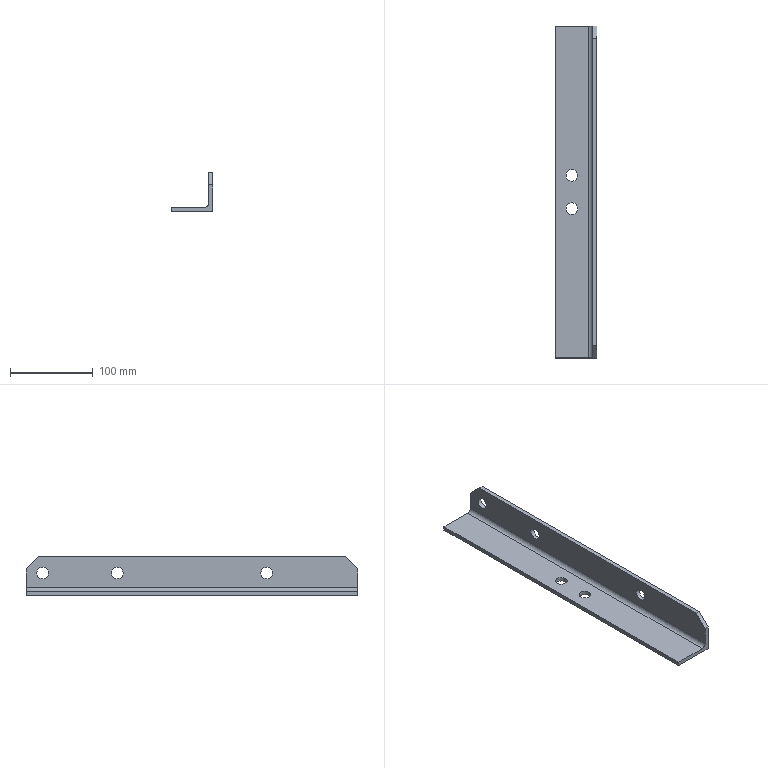Part | NX | features solid 2 | 1 solid | 16 faces | box 50 x 400 x 47 mm | volume 181173 mm3 | plane 10 | cylinder 6 | commonest cylinder face diameters 14 x5 10 x1
STEP:
#1=CARTESIAN_POINT('',(32.,860.,-22.059));
#2=VERTEX_POINT('',#1);
#3=CARTESIAN_POINT('',(25.,860.,-22.059));
#4=DIRECTION('',(0.,0.,-1.));
#5=DIRECTION('',(1.,0.,0.));
#6=AXIS2_PLACEMENT_3D('',#3,#4,#5);
#7=CIRCLE('',#6,7.);
#8=EDGE_CURVE('',#2,#2,#7,.F.);
#9=ORIENTED_EDGE('',*,*,#8,.F.);
#10=EDGE_LOOP('',(#9));
#11=FACE_BOUND('',#10,.T.);
#12=CARTESIAN_POINT('',(45.,1040.,-22.059));
#13=VERTEX_POINT('',#12);
#14=CARTESIAN_POINT('',(5.,1040.,-22.059));
#15=VERTEX_POINT('',#14);
#16=CARTESIAN_POINT('',(5.,1040.,-22.059));
#17=DIRECTION('',(-1.,0.,0.));
#18=VECTOR('',#17,1000.);
#19=LINE('',#16,#18);
#20=EDGE_CURVE('',#13,#15,#19,.T.);
#21=ORIENTED_EDGE('',*,*,#20,.T.);
#22=CARTESIAN_POINT('',(5.,640.,-22.059));
#23=VERTEX_POINT('',#22);
#24=CARTESIAN_POINT('',(5.,864.636,-22.059));
#25=DIRECTION('',(0.,1.,0.));
#26=VECTOR('',#25,1000.);
#27=LINE('',#24,#26);
#28=EDGE_CURVE('',#23,#15,#27,.T.);
#29=ORIENTED_EDGE('',*,*,#28,.F.);
#30=CARTESIAN_POINT('',(45.,640.,-22.059));
#31=VERTEX_POINT('',#30);
#32=CARTESIAN_POINT('',(50.,640.,-22.059));
#33=DIRECTION('',(1.,0.,0.));
#34=VECTOR('',#33,1000.);
#35=LINE('',#32,#34);
#36=EDGE_CURVE('',#23,#31,#35,.T.);
#37=ORIENTED_EDGE('',*,*,#36,.T.);
#38=CARTESIAN_POINT('',(45.,745.,-22.059));
#39=DIRECTION('',(0.,1.,0.));
#40=VECTOR('',#39,1000.);
#41=LINE('',#38,#40);
#42=EDGE_CURVE('',#13,#31,#41,.F.);
#43=ORIENTED_EDGE('',*,*,#42,.F.);
#44=EDGE_LOOP('',(#21,#29,#37,#43));
#45=FACE_BOUND('',#44,.T.);
#46=CARTESIAN_POINT('',(32.,820.,-22.059));
#47=VERTEX_POINT('',#46);
#48=CARTESIAN_POINT('',(25.,820.,-22.059));
#49=DIRECTION('',(0.,0.,-1.));
#50=DIRECTION('',(1.,0.,0.));
#51=AXIS2_PLACEMENT_3D('',#48,#49,#50);
#52=CIRCLE('',#51,7.);
#53=EDGE_CURVE('',#47,#47,#52,.F.);
#54=ORIENTED_EDGE('',*,*,#53,.F.);
#55=EDGE_LOOP('',(#54));
#56=FACE_BOUND('',#55,.T.);
#57=CARTESIAN_POINT('',(5.,862.805,-22.059));
#58=DIRECTION('',(0.,0.,1.));
#59=DIRECTION('',(0.,1.,0.));
#60=AXIS2_PLACEMENT_3D('',#57,#58,#59);
#61=PLANE('',#60);
#62=ADVANCED_FACE('',(#11,#45,#56),#61,.T.);
#63=CARTESIAN_POINT('',(18.,860.,-27.059));
#64=VERTEX_POINT('',#63);
#65=CARTESIAN_POINT('',(25.,860.,-27.059));
#66=DIRECTION('',(0.,0.,1.));
#67=DIRECTION('',(-1.,0.,0.));
#68=AXIS2_PLACEMENT_3D('',#65,#66,#67);
#69=CIRCLE('',#68,7.);
#70=EDGE_CURVE('',#64,#64,#69,.F.);
#71=ORIENTED_EDGE('',*,*,#70,.F.);
#72=EDGE_LOOP('',(#71));
#73=FACE_BOUND('',#72,.T.);
#74=CARTESIAN_POINT('',(5.,1040.,-27.059));
#75=VERTEX_POINT('',#74);
#76=CARTESIAN_POINT('',(55.,1040.,-27.059));
#77=VERTEX_POINT('',#76);
#78=CARTESIAN_POINT('',(50.,1040.,-27.059));
#79=DIRECTION('',(1.,0.,0.));
#80=VECTOR('',#79,1000.);
#81=LINE('',#78,#80);
#82=EDGE_CURVE('',#75,#77,#81,.T.);
#83=ORIENTED_EDGE('',*,*,#82,.T.);
#84=CARTESIAN_POINT('',(55.,640.,-27.059));
#85=VERTEX_POINT('',#84);
#86=CARTESIAN_POINT('',(55.,864.636,-27.059));
#87=DIRECTION('',(0.,1.,0.));
#88=VECTOR('',#87,1000.);
#89=LINE('',#86,#88);
#90=EDGE_CURVE('',#85,#77,#89,.T.);
#91=ORIENTED_EDGE('',*,*,#90,.F.);
#92=CARTESIAN_POINT('',(5.,640.,-27.059));
#93=VERTEX_POINT('',#92);
#94=CARTESIAN_POINT('',(50.,640.,-27.059));
#95=DIRECTION('',(-1.,0.,0.));
#96=VECTOR('',#95,1000.);
#97=LINE('',#94,#96);
#98=EDGE_CURVE('',#85,#93,#97,.T.);
#99=ORIENTED_EDGE('',*,*,#98,.T.);
#100=CARTESIAN_POINT('',(5.,862.5,-27.059));
#101=DIRECTION('',(0.,1.,0.));
#102=VECTOR('',#101,1000.);
#103=LINE('',#100,#102);
#104=EDGE_CURVE('',#93,#75,#103,.T.);
#105=ORIENTED_EDGE('',*,*,#104,.T.);
#106=EDGE_LOOP('',(#83,#91,#99,#105));
#107=FACE_BOUND('',#106,.T.);
#108=CARTESIAN_POINT('',(18.,820.,-27.059));
#109=VERTEX_POINT('',#108);
#110=CARTESIAN_POINT('',(25.,820.,-27.059));
#111=DIRECTION('',(0.,0.,1.));
#112=DIRECTION('',(-1.,0.,0.));
#113=AXIS2_PLACEMENT_3D('',#110,#111,#112);
#114=CIRCLE('',#113,7.);
#115=EDGE_CURVE('',#109,#109,#114,.F.);
#116=ORIENTED_EDGE('',*,*,#115,.F.);
#117=EDGE_LOOP('',(#116));
#118=FACE_BOUND('',#117,.T.);
#119=CARTESIAN_POINT('',(50.,862.5,-27.059));
#120=DIRECTION('',(0.,0.,-1.));
#121=DIRECTION('',(0.,-1.,0.));
#122=AXIS2_PLACEMENT_3D('',#119,#120,#121);
#123=PLANE('',#122);
#124=ADVANCED_FACE('',(#73,#107,#118),#123,.T.);
#125=CARTESIAN_POINT('',(50.,750.,-7.059));
#126=VERTEX_POINT('',#125);
#127=CARTESIAN_POINT('',(50.,750.,-0.05898));
#128=DIRECTION('',(-1.,0.,0.));
#129=DIRECTION('',(0.,0.,-1.));
#130=AXIS2_PLACEMENT_3D('',#127,#128,#129);
#131=CIRCLE('',#130,7.);
#132=EDGE_CURVE('',#126,#126,#131,.F.);
#133=ORIENTED_EDGE('',*,*,#132,.T.);
#134=EDGE_LOOP('',(#133));
#135=FACE_BOUND('',#134,.T.);
#136=CARTESIAN_POINT('',(50.,930.,-7.059));
#137=VERTEX_POINT('',#136);
#138=CARTESIAN_POINT('',(50.,930.,-0.05898));
#139=DIRECTION('',(-1.,0.,0.));
#140=DIRECTION('',(0.,0.,-1.));
#141=AXIS2_PLACEMENT_3D('',#138,#139,#140);
#142=CIRCLE('',#141,7.);
#143=EDGE_CURVE('',#137,#137,#142,.F.);
#144=ORIENTED_EDGE('',*,*,#143,.T.);
#145=EDGE_LOOP('',(#144));
#146=FACE_BOUND('',#145,.T.);
#147=CARTESIAN_POINT('',(50.,1040.,4.941));
#148=VERTEX_POINT('',#147);
#149=CARTESIAN_POINT('',(50.,1040.,-17.059));
#150=VERTEX_POINT('',#149);
#151=CARTESIAN_POINT('',(50.,1040.,7.941));
#152=DIRECTION('',(0.,0.,-1.));
#153=VECTOR('',#152,1000.);
#154=LINE('',#151,#153);
#155=EDGE_CURVE('',#148,#150,#154,.T.);
#156=ORIENTED_EDGE('',*,*,#155,.T.);
#157=CARTESIAN_POINT('',(50.,640.,-17.059));
#158=VERTEX_POINT('',#157);
#159=CARTESIAN_POINT('',(50.,1079.813,-17.059));
#160=DIRECTION('',(0.,1.,0.));
#161=VECTOR('',#160,1000.);
#162=LINE('',#159,#161);
#163=EDGE_CURVE('',#158,#150,#162,.T.);
#164=ORIENTED_EDGE('',*,*,#163,.F.);
#165=CARTESIAN_POINT('',(50.,640.,4.941));
#166=VERTEX_POINT('',#165);
#167=CARTESIAN_POINT('',(50.,640.,-0.05898));
#168=DIRECTION('',(0.,0.,1.));
#169=VECTOR('',#168,1000.);
#170=LINE('',#167,#169);
#171=EDGE_CURVE('',#158,#166,#170,.T.);
#172=ORIENTED_EDGE('',*,*,#171,.T.);
#173=CARTESIAN_POINT('',(50.,655.,19.941));
#174=VERTEX_POINT('',#173);
#175=CARTESIAN_POINT('',(50.,708.818,73.759));
#176=DIRECTION('',(0.,0.7071,0.7071));
#177=VECTOR('',#176,1000.);
#178=LINE('',#175,#177);
#179=EDGE_CURVE('',#174,#166,#178,.F.);
#180=ORIENTED_EDGE('',*,*,#179,.F.);
#181=CARTESIAN_POINT('',(50.,1025.,19.941));
#182=VERTEX_POINT('',#181);
#183=CARTESIAN_POINT('',(50.,864.636,19.941));
#184=DIRECTION('',(0.,1.,0.));
#185=VECTOR('',#184,1000.);
#186=LINE('',#183,#185);
#187=EDGE_CURVE('',#174,#182,#186,.T.);
#188=ORIENTED_EDGE('',*,*,#187,.T.);
#189=CARTESIAN_POINT('',(50.,950.818,94.123));
#190=DIRECTION('',(0.,-0.7071,0.7071));
#191=VECTOR('',#190,1000.);
#192=LINE('',#189,#191);
#193=EDGE_CURVE('',#148,#182,#192,.T.);
#194=ORIENTED_EDGE('',*,*,#193,.F.);
#195=EDGE_LOOP('',(#156,#164,#172,#180,#188,#194));
#196=FACE_BOUND('',#195,.T.);
#197=CARTESIAN_POINT('',(50.,1020.,6.941));
#198=VERTEX_POINT('',#197);
#199=CARTESIAN_POINT('',(50.,1020.,-0.05898));
#200=DIRECTION('',(1.,0.,0.));
#201=DIRECTION('',(0.,0.,1.));
#202=AXIS2_PLACEMENT_3D('',#199,#200,#201);
#203=CIRCLE('',#202,7.);
#204=EDGE_CURVE('',#198,#198,#203,.F.);
#205=ORIENTED_EDGE('',*,*,#204,.F.);
#206=EDGE_LOOP('',(#205));
#207=FACE_BOUND('',#206,.T.);
#208=CARTESIAN_POINT('',(50.,864.636,7.941));
#209=DIRECTION('',(-1.,0.,0.));
#210=DIRECTION('',(0.,0.,-1.));
#211=AXIS2_PLACEMENT_3D('',#208,#209,#210);
#212=PLANE('',#211);
#213=ADVANCED_FACE('',(#135,#146,#196,#207),#212,.T.);
#214=CARTESIAN_POINT('',(55.,750.,6.941));
#215=VERTEX_POINT('',#214);
#216=CARTESIAN_POINT('',(55.,750.,-0.05898));
#217=DIRECTION('',(1.,0.,0.));
#218=DIRECTION('',(0.,0.,1.));
#219=AXIS2_PLACEMENT_3D('',#216,#217,#218);
#220=CIRCLE('',#219,7.);
#221=EDGE_CURVE('',#215,#215,#220,.F.);
#222=ORIENTED_EDGE('',*,*,#221,.T.);
#223=EDGE_LOOP('',(#222));
#224=FACE_BOUND('',#223,.T.);
#225=CARTESIAN_POINT('',(55.,930.,6.941));
#226=VERTEX_POINT('',#225);
#227=CARTESIAN_POINT('',(55.,930.,-0.05898));
#228=DIRECTION('',(1.,0.,0.));
#229=DIRECTION('',(0.,0.,1.));
#230=AXIS2_PLACEMENT_3D('',#227,#228,#229);
#231=CIRCLE('',#230,7.);
#232=EDGE_CURVE('',#226,#226,#231,.F.);
#233=ORIENTED_EDGE('',*,*,#232,.T.);
#234=EDGE_LOOP('',(#233));
#235=FACE_BOUND('',#234,.T.);
#236=CARTESIAN_POINT('',(55.,655.,19.941));
#237=VERTEX_POINT('',#236);
#238=CARTESIAN_POINT('',(55.,1025.,19.941));
#239=VERTEX_POINT('',#238);
#240=CARTESIAN_POINT('',(55.,864.636,19.941));
#241=DIRECTION('',(0.,1.,0.));
#242=VECTOR('',#241,1000.);
#243=LINE('',#240,#242);
#244=EDGE_CURVE('',#237,#239,#243,.T.);
#245=ORIENTED_EDGE('',*,*,#244,.F.);
#246=CARTESIAN_POINT('',(55.,640.,4.941));
#247=VERTEX_POINT('',#246);
#248=CARTESIAN_POINT('',(55.,708.818,73.759));
#249=DIRECTION('',(0.,-0.7071,-0.7071));
#250=VECTOR('',#249,1000.);
#251=LINE('',#248,#250);
#252=EDGE_CURVE('',#247,#237,#251,.F.);
#253=ORIENTED_EDGE('',*,*,#252,.F.);
#254=CARTESIAN_POINT('',(55.,640.,-0.05898));
#255=DIRECTION('',(0.,0.,-1.));
#256=VECTOR('',#255,1000.);
#257=LINE('',#254,#256);
#258=EDGE_CURVE('',#247,#85,#257,.T.);
#259=ORIENTED_EDGE('',*,*,#258,.T.);
#260=ORIENTED_EDGE('',*,*,#90,.T.);
#261=CARTESIAN_POINT('',(55.,1040.,4.941));
#262=VERTEX_POINT('',#261);
#263=CARTESIAN_POINT('',(55.,1040.,7.941));
#264=DIRECTION('',(0.,0.,1.));
#265=VECTOR('',#264,1000.);
#266=LINE('',#263,#265);
#267=EDGE_CURVE('',#77,#262,#266,.T.);
#268=ORIENTED_EDGE('',*,*,#267,.T.);
#269=CARTESIAN_POINT('',(55.,950.818,94.123));
#270=DIRECTION('',(0.,0.7071,-0.7071));
#271=VECTOR('',#270,1000.);
#272=LINE('',#269,#271);
#273=EDGE_CURVE('',#239,#262,#272,.T.);
#274=ORIENTED_EDGE('',*,*,#273,.F.);
#275=EDGE_LOOP('',(#245,#253,#259,#260,#268,#274));
#276=FACE_BOUND('',#275,.T.);
#277=CARTESIAN_POINT('',(55.,1020.,-7.059));
#278=VERTEX_POINT('',#277);
#279=CARTESIAN_POINT('',(55.,1020.,-0.05898));
#280=DIRECTION('',(-1.,0.,0.));
#281=DIRECTION('',(0.,0.,-1.));
#282=AXIS2_PLACEMENT_3D('',#279,#280,#281);
#283=CIRCLE('',#282,7.);
#284=EDGE_CURVE('',#278,#278,#283,.T.);
#285=ORIENTED_EDGE('',*,*,#284,.T.);
#286=EDGE_LOOP('',(#285));
#287=FACE_BOUND('',#286,.T.);
#288=CARTESIAN_POINT('',(55.,864.636,7.941));
#289=DIRECTION('',(1.,0.,0.));
#290=DIRECTION('',(0.,0.,1.));
#291=AXIS2_PLACEMENT_3D('',#288,#289,#290);
#292=PLANE('',#291);
#293=ADVANCED_FACE('',(#224,#235,#276,#287),#292,.T.);
#294=ORIENTED_EDGE('',*,*,#187,.F.);
#295=CARTESIAN_POINT('',(45.,655.,19.941));
#296=DIRECTION('',(-1.,0.,0.));
#297=VECTOR('',#296,1000.);
#298=LINE('',#295,#297);
#299=EDGE_CURVE('',#237,#174,#298,.T.);
#300=ORIENTED_EDGE('',*,*,#299,.F.);
#301=ORIENTED_EDGE('',*,*,#244,.T.);
#302=CARTESIAN_POINT('',(55.,1025.,19.941));
#303=DIRECTION('',(1.,0.,0.));
#304=VECTOR('',#303,1000.);
#305=LINE('',#302,#304);
#306=EDGE_CURVE('',#182,#239,#305,.T.);
#307=ORIENTED_EDGE('',*,*,#306,.F.);
#308=EDGE_LOOP('',(#294,#300,#301,#307));
#309=FACE_BOUND('',#308,.T.);
#310=CARTESIAN_POINT('',(45.,864.636,19.941));
#311=DIRECTION('',(0.,0.,1.));
#312=DIRECTION('',(0.,1.,0.));
#313=AXIS2_PLACEMENT_3D('',#310,#311,#312);
#314=PLANE('',#313);
#315=ADVANCED_FACE('',(#309),#314,.T.);
#316=ORIENTED_EDGE('',*,*,#42,.T.);
#317=CARTESIAN_POINT('',(45.,640.,-17.059));
#318=DIRECTION('',(0.,1.,0.));
#319=DIRECTION('',(-0.9063,0.,-0.4226));
#320=AXIS2_PLACEMENT_3D('',#317,#318,#319);
#321=CIRCLE('',#320,5.);
#322=EDGE_CURVE('',#158,#31,#321,.T.);
#323=ORIENTED_EDGE('',*,*,#322,.F.);
#324=ORIENTED_EDGE('',*,*,#163,.T.);
#325=CARTESIAN_POINT('',(45.,1040.,-17.059));
#326=DIRECTION('',(0.,1.,0.));
#327=DIRECTION('',(-0.4226,0.,0.9063));
#328=AXIS2_PLACEMENT_3D('',#325,#326,#327);
#329=CIRCLE('',#328,5.);
#330=EDGE_CURVE('',#13,#150,#329,.F.);
#331=ORIENTED_EDGE('',*,*,#330,.F.);
#332=EDGE_LOOP('',(#316,#323,#324,#331));
#333=FACE_BOUND('',#332,.T.);
#334=CARTESIAN_POINT('',(45.,864.636,-17.059));
#335=DIRECTION('',(0.,-1.,0.));
#336=DIRECTION('',(0.,0.,-1.));
#337=AXIS2_PLACEMENT_3D('',#334,#335,#336);
#338=CYLINDRICAL_SURFACE('',#337,5.);
#339=ADVANCED_FACE('',(#333),#338,.F.);
#340=CARTESIAN_POINT('',(5.,1040.,7.941));
#341=DIRECTION('',(0.,0.,-1.));
#342=VECTOR('',#341,1000.);
#343=LINE('',#340,#342);
#344=EDGE_CURVE('',#15,#75,#343,.T.);
#345=ORIENTED_EDGE('',*,*,#344,.T.);
#346=ORIENTED_EDGE('',*,*,#104,.F.);
#347=CARTESIAN_POINT('',(5.,640.,-0.05898));
#348=DIRECTION('',(0.,0.,1.));
#349=VECTOR('',#348,1000.);
#350=LINE('',#347,#349);
#351=EDGE_CURVE('',#93,#23,#350,.T.);
#352=ORIENTED_EDGE('',*,*,#351,.T.);
#353=ORIENTED_EDGE('',*,*,#28,.T.);
#354=EDGE_LOOP('',(#345,#346,#352,#353));
#355=FACE_BOUND('',#354,.T.);
#356=CARTESIAN_POINT('',(5.,864.636,7.941));
#357=DIRECTION('',(-1.,0.,0.));
#358=DIRECTION('',(0.,0.,-1.));
#359=AXIS2_PLACEMENT_3D('',#356,#357,#358);
#360=PLANE('',#359);
#361=ADVANCED_FACE('',(#355),#360,.T.);
#362=ORIENTED_EDGE('',*,*,#143,.F.);
#363=EDGE_LOOP('',(#362));
#364=FACE_BOUND('',#363,.T.);
#365=ORIENTED_EDGE('',*,*,#232,.F.);
#366=EDGE_LOOP('',(#365));
#367=FACE_BOUND('',#366,.T.);
#368=CARTESIAN_POINT('',(25.,930.,-0.05898));
#369=DIRECTION('',(1.,0.,0.));
#370=DIRECTION('',(0.,1.,0.));
#371=AXIS2_PLACEMENT_3D('',#368,#369,#370);
#372=CYLINDRICAL_SURFACE('',#371,7.);
#373=ADVANCED_FACE('',(#364,#367),#372,.F.);
#374=ORIENTED_EDGE('',*,*,#267,.F.);
#375=ORIENTED_EDGE('',*,*,#82,.F.);
#376=ORIENTED_EDGE('',*,*,#344,.F.);
#377=ORIENTED_EDGE('',*,*,#20,.F.);
#378=ORIENTED_EDGE('',*,*,#330,.T.);
#379=ORIENTED_EDGE('',*,*,#155,.F.);
#380=CARTESIAN_POINT('',(50.,1040.,4.941));
#381=DIRECTION('',(-1.,0.,0.));
#382=VECTOR('',#381,1000.);
#383=LINE('',#380,#382);
#384=EDGE_CURVE('',#262,#148,#383,.T.);
#385=ORIENTED_EDGE('',*,*,#384,.F.);
#386=EDGE_LOOP('',(#374,#375,#376,#377,#378,#379,#385));
#387=FACE_BOUND('',#386,.T.);
#388=CARTESIAN_POINT('',(633.203,1040.,86.834));
#389=DIRECTION('',(0.,-1.,0.));
#390=DIRECTION('',(-0.4226,0.,0.9063));
#391=AXIS2_PLACEMENT_3D('',#388,#389,#390);
#392=PLANE('',#391);
#393=ADVANCED_FACE('',(#387),#392,.F.);
#394=ORIENTED_EDGE('',*,*,#171,.F.);
#395=ORIENTED_EDGE('',*,*,#322,.T.);
#396=ORIENTED_EDGE('',*,*,#36,.F.);
#397=ORIENTED_EDGE('',*,*,#351,.F.);
#398=ORIENTED_EDGE('',*,*,#98,.F.);
#399=ORIENTED_EDGE('',*,*,#258,.F.);
#400=CARTESIAN_POINT('',(50.,640.,4.941));
#401=DIRECTION('',(1.,0.,0.));
#402=VECTOR('',#401,1000.);
#403=LINE('',#400,#402);
#404=EDGE_CURVE('',#166,#247,#403,.T.);
#405=ORIENTED_EDGE('',*,*,#404,.F.);
#406=EDGE_LOOP('',(#394,#395,#396,#397,#398,#399,#405));
#407=FACE_BOUND('',#406,.T.);
#408=CARTESIAN_POINT('',(50.,640.,-0.05898));
#409=DIRECTION('',(0.,-1.,0.));
#410=DIRECTION('',(0.9063,0.,-0.4226));
#411=AXIS2_PLACEMENT_3D('',#408,#409,#410);
#412=PLANE('',#411);
#413=ADVANCED_FACE('',(#407),#412,.T.);
#414=ORIENTED_EDGE('',*,*,#132,.F.);
#415=EDGE_LOOP('',(#414));
#416=FACE_BOUND('',#415,.T.);
#417=ORIENTED_EDGE('',*,*,#221,.F.);
#418=EDGE_LOOP('',(#417));
#419=FACE_BOUND('',#418,.T.);
#420=CARTESIAN_POINT('',(25.,750.,-0.05898));
#421=DIRECTION('',(1.,0.,0.));
#422=DIRECTION('',(0.,1.,0.));
#423=AXIS2_PLACEMENT_3D('',#420,#421,#422);
#424=CYLINDRICAL_SURFACE('',#423,7.);
#425=ADVANCED_FACE('',(#416,#419),#424,.F.);
#426=ORIENTED_EDGE('',*,*,#204,.T.);
#427=EDGE_LOOP('',(#426));
#428=FACE_BOUND('',#427,.T.);
#429=ORIENTED_EDGE('',*,*,#284,.F.);
#430=EDGE_LOOP('',(#429));
#431=FACE_BOUND('',#430,.T.);
#432=CARTESIAN_POINT('',(25.,1020.,-0.05898));
#433=DIRECTION('',(1.,0.,0.));
#434=DIRECTION('',(0.,1.,0.));
#435=AXIS2_PLACEMENT_3D('',#432,#433,#434);
#436=CYLINDRICAL_SURFACE('',#435,7.);
#437=ADVANCED_FACE('',(#428,#431),#436,.F.);
#438=ORIENTED_EDGE('',*,*,#273,.T.);
#439=ORIENTED_EDGE('',*,*,#384,.T.);
#440=ORIENTED_EDGE('',*,*,#193,.T.);
#441=ORIENTED_EDGE('',*,*,#306,.T.);
#442=EDGE_LOOP('',(#438,#439,#440,#441));
#443=FACE_BOUND('',#442,.T.);
#444=CARTESIAN_POINT('',(633.203,1040.,4.941));
#445=DIRECTION('',(0.,0.7071,0.7071));
#446=DIRECTION('',(0.3131,0.6715,-0.6715));
#447=AXIS2_PLACEMENT_3D('',#444,#445,#446);
#448=PLANE('',#447);
#449=ADVANCED_FACE('',(#443),#448,.T.);
#450=ORIENTED_EDGE('',*,*,#179,.T.);
#451=ORIENTED_EDGE('',*,*,#404,.T.);
#452=ORIENTED_EDGE('',*,*,#252,.T.);
#453=ORIENTED_EDGE('',*,*,#299,.T.);
#454=EDGE_LOOP('',(#450,#451,#452,#453));
#455=FACE_BOUND('',#454,.T.);
#456=CARTESIAN_POINT('',(50.,640.,4.941));
#457=DIRECTION('',(0.,0.7071,-0.7071));
#458=DIRECTION('',(0.3131,-0.6715,-0.6715));
#459=AXIS2_PLACEMENT_3D('',#456,#457,#458);
#460=PLANE('',#459);
#461=ADVANCED_FACE('',(#455),#460,.F.);
#462=ORIENTED_EDGE('',*,*,#8,.T.);
#463=EDGE_LOOP('',(#462));
#464=FACE_BOUND('',#463,.T.);
#465=ORIENTED_EDGE('',*,*,#70,.T.);
#466=EDGE_LOOP('',(#465));
#467=FACE_BOUND('',#466,.T.);
#468=CARTESIAN_POINT('',(25.,860.,-72.021));
#469=DIRECTION('',(0.,0.,1.));
#470=DIRECTION('',(1.,0.,0.));
#471=AXIS2_PLACEMENT_3D('',#468,#469,#470);
#472=CYLINDRICAL_SURFACE('',#471,7.);
#473=ADVANCED_FACE('',(#464,#467),#472,.F.);
#474=ORIENTED_EDGE('',*,*,#53,.T.);
#475=EDGE_LOOP('',(#474));
#476=FACE_BOUND('',#475,.T.);
#477=ORIENTED_EDGE('',*,*,#115,.T.);
#478=EDGE_LOOP('',(#477));
#479=FACE_BOUND('',#478,.T.);
#480=CARTESIAN_POINT('',(25.,820.,-72.021));
#481=DIRECTION('',(0.,0.,1.));
#482=DIRECTION('',(1.,0.,0.));
#483=AXIS2_PLACEMENT_3D('',#480,#481,#482);
#484=CYLINDRICAL_SURFACE('',#483,7.);
#485=ADVANCED_FACE('',(#476,#479),#484,.F.);
#486=CLOSED_SHELL('',(#62,#124,#213,#293,#315,#339,#361,#373,#393,#413,#425,#437,#449,#461,#473,#485));
#487=MANIFOLD_SOLID_BREP('',#486);
#488=(LENGTH_UNIT()NAMED_UNIT(*)SI_UNIT(.MILLI.,.METRE.));
#489=UNCERTAINTY_MEASURE_WITH_UNIT(LENGTH_MEASURE(0.00001),#488,'','');
#490=(NAMED_UNIT(*)PLANE_ANGLE_UNIT()SI_UNIT($,.RADIAN.));
#491=(NAMED_UNIT(*)SI_UNIT($,.STERADIAN.)SOLID_ANGLE_UNIT());
#492=(GEOMETRIC_REPRESENTATION_CONTEXT(3)GLOBAL_UNCERTAINTY_ASSIGNED_CONTEXT((#489))GLOBAL_UNIT_ASSIGNED_CONTEXT((#488,#490,#491))REPRESENTATION_CONTEXT('',''));
#493=ADVANCED_BREP_SHAPE_REPRESENTATION('',(#487),#492);